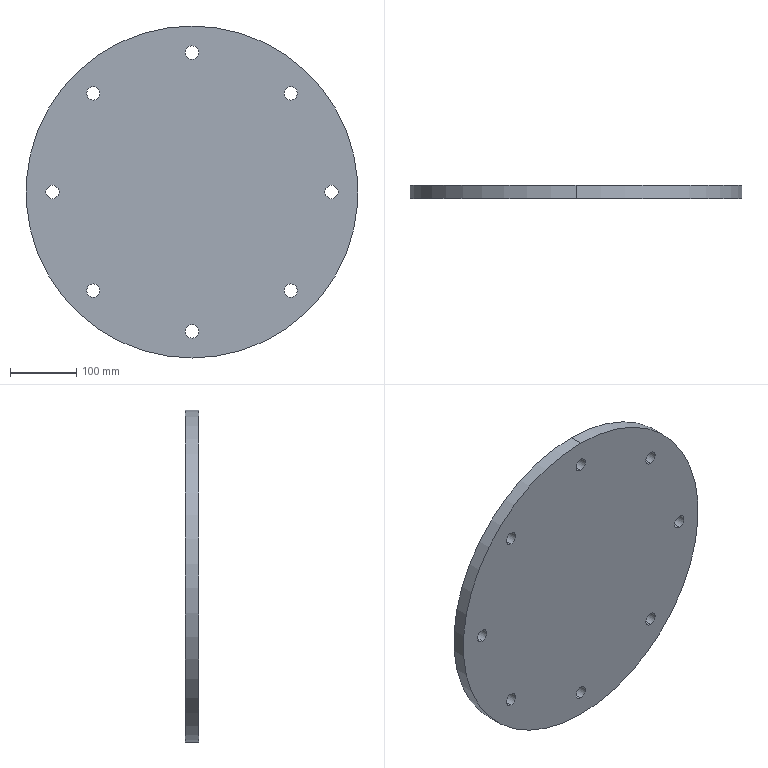Part | STEP file | 113_4 | 1 solid | 20 faces | box 500 x 20 x 500 mm | volume 3876725 mm3 | cylinder 18 | plane 2 | commonest cylinder face diameters 20 x16 500 x2